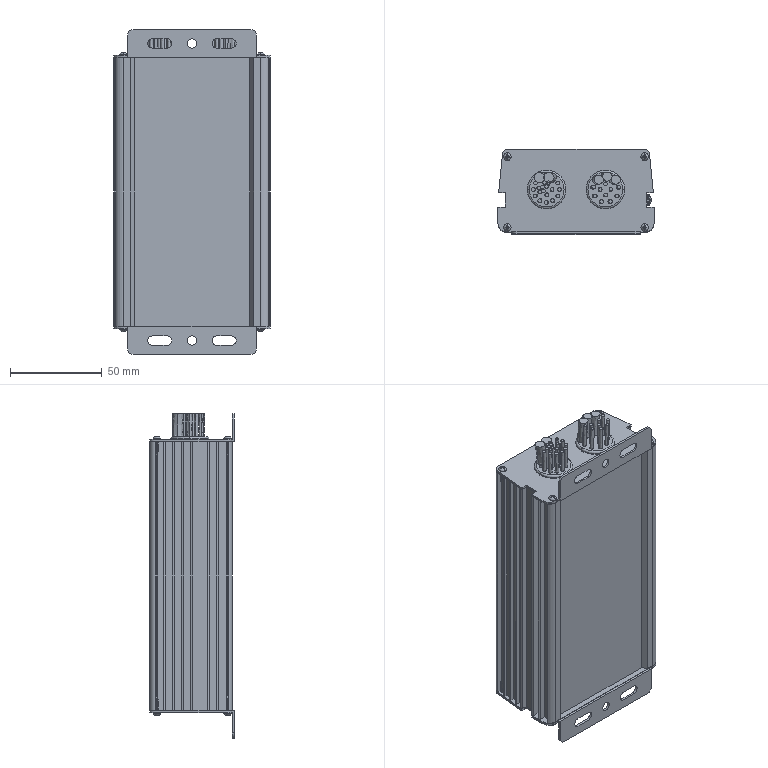Part | SolidWorks | features BaseBody 49 | 49 solids | 2216 faces | box 85.012 x 46.209 x 176.601 mm | volume 88332 mm3 | cylinder 1087 | plane 665 | spline 289 | cone 109 | torus 40 | sphere 26 | commonest cylinder face diameters 3 x318 2.35 x205 1.575 x176 2.17 x152 2 x98 2.002 x36